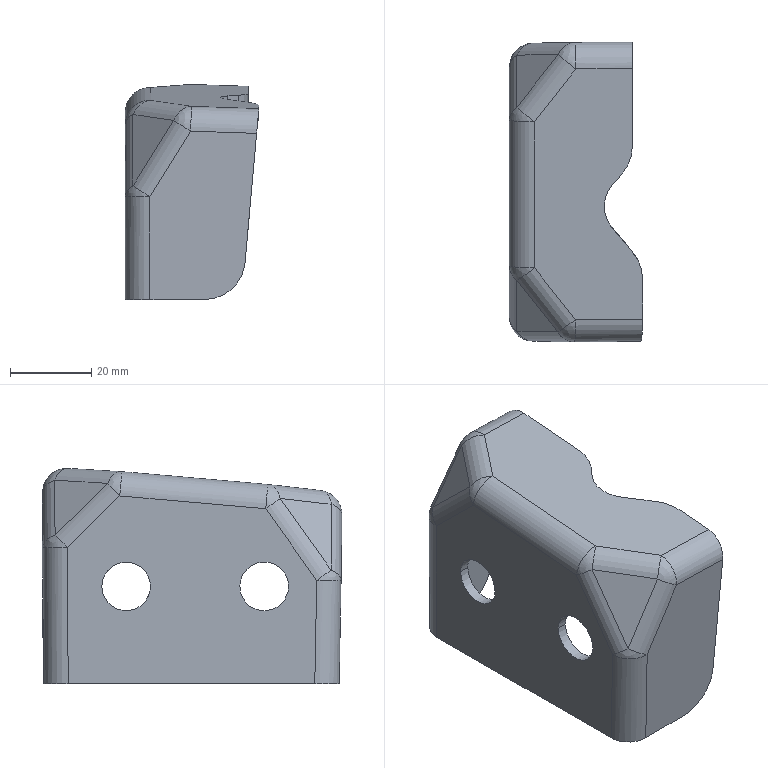Part | 1 solid | 70 faces | box 32.815 x 73.854 x 52.988 mm | volume 18099 mm3 | cylinder 27 | spline 22 | sphere 12 | plane 9 | commonest cylinder face diameters 12 x15 7 x11 16 x1